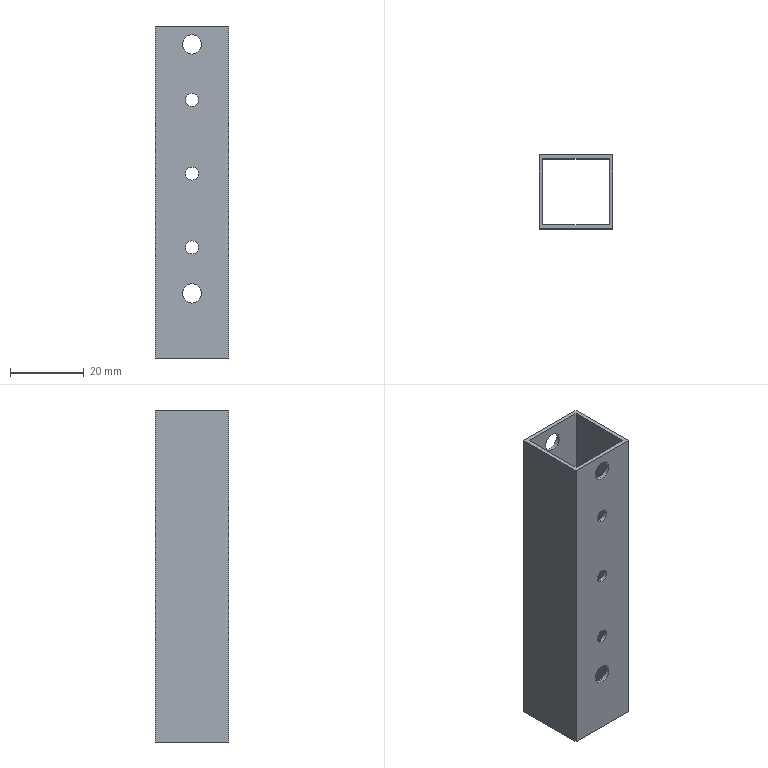Part | SolidWorks | features BaseBody 1 | 1 solid | 30 faces | box 20 x 20 x 90 mm | volume 6697 mm3 | cylinder 20 | plane 10 | commonest cylinder face diameters 3.5 x12 5.2 x8
STEP:
#1=CARTESIAN_POINT('',(0.,9.,68.25));
#2=VERTEX_POINT('',#1);
#3=CARTESIAN_POINT('',(0.,9.,71.75));
#4=VERTEX_POINT('',#3);
#5=CARTESIAN_POINT('',(0.,9.,70.));
#6=DIRECTION('',(0.,1.,0.));
#7=DIRECTION('',(0.,0.,1.));
#8=AXIS2_PLACEMENT_3D('',#5,#6,#7);
#9=CIRCLE('',#8,1.75);
#10=EDGE_CURVE('',#2,#4,#9,.T.);
#11=ORIENTED_EDGE('',*,*,#10,.F.);
#12=CARTESIAN_POINT('',(0.,10.,68.25));
#13=VERTEX_POINT('',#12);
#14=CARTESIAN_POINT('',(0.,-80.,68.25));
#15=DIRECTION('',(0.,1.,0.));
#16=VECTOR('',#15,1000.);
#17=LINE('',#14,#16);
#18=EDGE_CURVE('',#2,#13,#17,.T.);
#19=ORIENTED_EDGE('',*,*,#18,.T.);
#20=CARTESIAN_POINT('',(0.,10.,71.75));
#21=VERTEX_POINT('',#20);
#22=CARTESIAN_POINT('',(0.,10.,70.));
#23=DIRECTION('',(0.,1.,0.));
#24=DIRECTION('',(0.,0.,1.));
#25=AXIS2_PLACEMENT_3D('',#22,#23,#24);
#26=CIRCLE('',#25,1.75);
#27=EDGE_CURVE('',#13,#21,#26,.T.);
#28=ORIENTED_EDGE('',*,*,#27,.T.);
#29=CARTESIAN_POINT('',(0.,-80.,71.75));
#30=DIRECTION('',(0.,1.,0.));
#31=VECTOR('',#30,1000.);
#32=LINE('',#29,#31);
#33=EDGE_CURVE('',#4,#21,#32,.T.);
#34=ORIENTED_EDGE('',*,*,#33,.F.);
#35=EDGE_LOOP('',(#11,#19,#28,#34));
#36=FACE_OUTER_BOUND('',#35,.T.);
#37=CARTESIAN_POINT('',(0.,-80.,70.));
#38=DIRECTION('',(0.,1.,0.));
#39=DIRECTION('',(0.,0.,1.));
#40=AXIS2_PLACEMENT_3D('',#37,#38,#39);
#41=CYLINDRICAL_SURFACE('',#40,1.75);
#42=ADVANCED_FACE('',(#36),#41,.F.);
#43=CARTESIAN_POINT('',(0.,9.,14.9));
#44=VERTEX_POINT('',#43);
#45=CARTESIAN_POINT('',(0.,9.,20.1));
#46=VERTEX_POINT('',#45);
#47=CARTESIAN_POINT('',(0.,9.,17.5));
#48=DIRECTION('',(0.,1.,0.));
#49=DIRECTION('',(0.,0.,1.));
#50=AXIS2_PLACEMENT_3D('',#47,#48,#49);
#51=CIRCLE('',#50,2.6);
#52=EDGE_CURVE('',#44,#46,#51,.T.);
#53=ORIENTED_EDGE('',*,*,#52,.F.);
#54=CARTESIAN_POINT('',(0.,10.,14.9));
#55=VERTEX_POINT('',#54);
#56=CARTESIAN_POINT('',(0.,-80.,14.9));
#57=DIRECTION('',(0.,1.,0.));
#58=VECTOR('',#57,1000.);
#59=LINE('',#56,#58);
#60=EDGE_CURVE('',#44,#55,#59,.T.);
#61=ORIENTED_EDGE('',*,*,#60,.T.);
#62=CARTESIAN_POINT('',(0.,10.,20.1));
#63=VERTEX_POINT('',#62);
#64=CARTESIAN_POINT('',(0.,10.,17.5));
#65=DIRECTION('',(0.,1.,0.));
#66=DIRECTION('',(0.,0.,1.));
#67=AXIS2_PLACEMENT_3D('',#64,#65,#66);
#68=CIRCLE('',#67,2.6);
#69=EDGE_CURVE('',#55,#63,#68,.T.);
#70=ORIENTED_EDGE('',*,*,#69,.T.);
#71=CARTESIAN_POINT('',(0.,-80.,20.1));
#72=DIRECTION('',(0.,1.,0.));
#73=VECTOR('',#72,1000.);
#74=LINE('',#71,#73);
#75=EDGE_CURVE('',#46,#63,#74,.T.);
#76=ORIENTED_EDGE('',*,*,#75,.F.);
#77=EDGE_LOOP('',(#53,#61,#70,#76));
#78=FACE_OUTER_BOUND('',#77,.T.);
#79=CARTESIAN_POINT('',(0.,-80.,17.5));
#80=DIRECTION('',(0.,1.,0.));
#81=DIRECTION('',(0.,0.,1.));
#82=AXIS2_PLACEMENT_3D('',#79,#80,#81);
#83=CYLINDRICAL_SURFACE('',#82,2.6);
#84=ADVANCED_FACE('',(#78),#83,.F.);
#85=CARTESIAN_POINT('',(0.,9.,48.25));
#86=VERTEX_POINT('',#85);
#87=CARTESIAN_POINT('',(0.,9.,51.75));
#88=VERTEX_POINT('',#87);
#89=CARTESIAN_POINT('',(0.,9.,50.));
#90=DIRECTION('',(0.,1.,0.));
#91=DIRECTION('',(0.,0.,1.));
#92=AXIS2_PLACEMENT_3D('',#89,#90,#91);
#93=CIRCLE('',#92,1.75);
#94=EDGE_CURVE('',#86,#88,#93,.T.);
#95=ORIENTED_EDGE('',*,*,#94,.F.);
#96=CARTESIAN_POINT('',(0.,10.,48.25));
#97=VERTEX_POINT('',#96);
#98=CARTESIAN_POINT('',(0.,-80.,48.25));
#99=DIRECTION('',(0.,1.,0.));
#100=VECTOR('',#99,1000.);
#101=LINE('',#98,#100);
#102=EDGE_CURVE('',#86,#97,#101,.T.);
#103=ORIENTED_EDGE('',*,*,#102,.T.);
#104=CARTESIAN_POINT('',(0.,10.,51.75));
#105=VERTEX_POINT('',#104);
#106=CARTESIAN_POINT('',(0.,10.,50.));
#107=DIRECTION('',(0.,1.,0.));
#108=DIRECTION('',(0.,0.,1.));
#109=AXIS2_PLACEMENT_3D('',#106,#107,#108);
#110=CIRCLE('',#109,1.75);
#111=EDGE_CURVE('',#97,#105,#110,.T.);
#112=ORIENTED_EDGE('',*,*,#111,.T.);
#113=CARTESIAN_POINT('',(0.,-80.,51.75));
#114=DIRECTION('',(0.,1.,0.));
#115=VECTOR('',#114,1000.);
#116=LINE('',#113,#115);
#117=EDGE_CURVE('',#88,#105,#116,.T.);
#118=ORIENTED_EDGE('',*,*,#117,.F.);
#119=EDGE_LOOP('',(#95,#103,#112,#118));
#120=FACE_OUTER_BOUND('',#119,.T.);
#121=CARTESIAN_POINT('',(0.,-80.,50.));
#122=DIRECTION('',(0.,1.,0.));
#123=DIRECTION('',(0.,0.,1.));
#124=AXIS2_PLACEMENT_3D('',#121,#122,#123);
#125=CYLINDRICAL_SURFACE('',#124,1.75);
#126=ADVANCED_FACE('',(#120),#125,.F.);
#127=CARTESIAN_POINT('',(0.,9.,28.25));
#128=VERTEX_POINT('',#127);
#129=CARTESIAN_POINT('',(0.,9.,31.75));
#130=VERTEX_POINT('',#129);
#131=CARTESIAN_POINT('',(0.,9.,30.));
#132=DIRECTION('',(0.,1.,0.));
#133=DIRECTION('',(0.,0.,1.));
#134=AXIS2_PLACEMENT_3D('',#131,#132,#133);
#135=CIRCLE('',#134,1.75);
#136=EDGE_CURVE('',#128,#130,#135,.T.);
#137=ORIENTED_EDGE('',*,*,#136,.F.);
#138=CARTESIAN_POINT('',(0.,10.,28.25));
#139=VERTEX_POINT('',#138);
#140=CARTESIAN_POINT('',(0.,-80.,28.25));
#141=DIRECTION('',(0.,1.,0.));
#142=VECTOR('',#141,1000.);
#143=LINE('',#140,#142);
#144=EDGE_CURVE('',#128,#139,#143,.T.);
#145=ORIENTED_EDGE('',*,*,#144,.T.);
#146=CARTESIAN_POINT('',(0.,10.,31.75));
#147=VERTEX_POINT('',#146);
#148=CARTESIAN_POINT('',(0.,10.,30.));
#149=DIRECTION('',(0.,1.,0.));
#150=DIRECTION('',(0.,0.,1.));
#151=AXIS2_PLACEMENT_3D('',#148,#149,#150);
#152=CIRCLE('',#151,1.75);
#153=EDGE_CURVE('',#139,#147,#152,.T.);
#154=ORIENTED_EDGE('',*,*,#153,.T.);
#155=CARTESIAN_POINT('',(0.,-80.,31.75));
#156=DIRECTION('',(0.,1.,0.));
#157=VECTOR('',#156,1000.);
#158=LINE('',#155,#157);
#159=EDGE_CURVE('',#130,#147,#158,.T.);
#160=ORIENTED_EDGE('',*,*,#159,.F.);
#161=EDGE_LOOP('',(#137,#145,#154,#160));
#162=FACE_OUTER_BOUND('',#161,.T.);
#163=CARTESIAN_POINT('',(0.,-80.,30.));
#164=DIRECTION('',(0.,1.,0.));
#165=DIRECTION('',(0.,0.,1.));
#166=AXIS2_PLACEMENT_3D('',#163,#164,#165);
#167=CYLINDRICAL_SURFACE('',#166,1.75);
#168=ADVANCED_FACE('',(#162),#167,.F.);
#169=CARTESIAN_POINT('',(0.,9.,82.4));
#170=VERTEX_POINT('',#169);
#171=CARTESIAN_POINT('',(0.,9.,87.6));
#172=VERTEX_POINT('',#171);
#173=CARTESIAN_POINT('',(0.,9.,85.));
#174=DIRECTION('',(0.,1.,0.));
#175=DIRECTION('',(0.,0.,1.));
#176=AXIS2_PLACEMENT_3D('',#173,#174,#175);
#177=CIRCLE('',#176,2.6);
#178=EDGE_CURVE('',#170,#172,#177,.T.);
#179=ORIENTED_EDGE('',*,*,#178,.F.);
#180=CARTESIAN_POINT('',(0.,10.,82.4));
#181=VERTEX_POINT('',#180);
#182=CARTESIAN_POINT('',(0.,-80.,82.4));
#183=DIRECTION('',(0.,1.,0.));
#184=VECTOR('',#183,1000.);
#185=LINE('',#182,#184);
#186=EDGE_CURVE('',#170,#181,#185,.T.);
#187=ORIENTED_EDGE('',*,*,#186,.T.);
#188=CARTESIAN_POINT('',(0.,10.,87.6));
#189=VERTEX_POINT('',#188);
#190=CARTESIAN_POINT('',(0.,10.,85.));
#191=DIRECTION('',(0.,1.,0.));
#192=DIRECTION('',(0.,0.,1.));
#193=AXIS2_PLACEMENT_3D('',#190,#191,#192);
#194=CIRCLE('',#193,2.6);
#195=EDGE_CURVE('',#181,#189,#194,.T.);
#196=ORIENTED_EDGE('',*,*,#195,.T.);
#197=CARTESIAN_POINT('',(0.,-80.,87.6));
#198=DIRECTION('',(0.,1.,0.));
#199=VECTOR('',#198,1000.);
#200=LINE('',#197,#199);
#201=EDGE_CURVE('',#172,#189,#200,.T.);
#202=ORIENTED_EDGE('',*,*,#201,.F.);
#203=EDGE_LOOP('',(#179,#187,#196,#202));
#204=FACE_OUTER_BOUND('',#203,.T.);
#205=CARTESIAN_POINT('',(0.,-80.,85.));
#206=DIRECTION('',(0.,1.,0.));
#207=DIRECTION('',(0.,0.,1.));
#208=AXIS2_PLACEMENT_3D('',#205,#206,#207);
#209=CYLINDRICAL_SURFACE('',#208,2.6);
#210=ADVANCED_FACE('',(#204),#209,.F.);
#211=CARTESIAN_POINT('',(0.,-10.,71.75));
#212=VERTEX_POINT('',#211);
#213=CARTESIAN_POINT('',(0.,-10.,68.25));
#214=VERTEX_POINT('',#213);
#215=CARTESIAN_POINT('',(0.,-10.,70.));
#216=DIRECTION('',(0.,-1.,0.));
#217=DIRECTION('',(0.,0.,1.));
#218=AXIS2_PLACEMENT_3D('',#215,#216,#217);
#219=CIRCLE('',#218,1.75);
#220=EDGE_CURVE('',#212,#214,#219,.T.);
#221=ORIENTED_EDGE('',*,*,#220,.T.);
#222=CARTESIAN_POINT('',(0.,-9.,68.25));
#223=VERTEX_POINT('',#222);
#224=CARTESIAN_POINT('',(0.,-80.,68.25));
#225=DIRECTION('',(0.,1.,0.));
#226=VECTOR('',#225,1000.);
#227=LINE('',#224,#226);
#228=EDGE_CURVE('',#214,#223,#227,.T.);
#229=ORIENTED_EDGE('',*,*,#228,.T.);
#230=CARTESIAN_POINT('',(0.,-9.,71.75));
#231=VERTEX_POINT('',#230);
#232=CARTESIAN_POINT('',(0.,-9.,70.));
#233=DIRECTION('',(0.,-1.,0.));
#234=DIRECTION('',(0.,0.,1.));
#235=AXIS2_PLACEMENT_3D('',#232,#233,#234);
#236=CIRCLE('',#235,1.75);
#237=EDGE_CURVE('',#231,#223,#236,.T.);
#238=ORIENTED_EDGE('',*,*,#237,.F.);
#239=CARTESIAN_POINT('',(0.,-80.,71.75));
#240=DIRECTION('',(0.,1.,0.));
#241=VECTOR('',#240,1000.);
#242=LINE('',#239,#241);
#243=EDGE_CURVE('',#212,#231,#242,.T.);
#244=ORIENTED_EDGE('',*,*,#243,.F.);
#245=EDGE_LOOP('',(#221,#229,#238,#244));
#246=FACE_OUTER_BOUND('',#245,.T.);
#247=CARTESIAN_POINT('',(0.,-80.,70.));
#248=DIRECTION('',(0.,1.,0.));
#249=DIRECTION('',(0.,0.,1.));
#250=AXIS2_PLACEMENT_3D('',#247,#248,#249);
#251=CYLINDRICAL_SURFACE('',#250,1.75);
#252=ADVANCED_FACE('',(#246),#251,.F.);
#253=CARTESIAN_POINT('',(0.,-10.,20.1));
#254=VERTEX_POINT('',#253);
#255=CARTESIAN_POINT('',(0.,-10.,14.9));
#256=VERTEX_POINT('',#255);
#257=CARTESIAN_POINT('',(0.,-10.,17.5));
#258=DIRECTION('',(0.,-1.,0.));
#259=DIRECTION('',(0.,0.,1.));
#260=AXIS2_PLACEMENT_3D('',#257,#258,#259);
#261=CIRCLE('',#260,2.6);
#262=EDGE_CURVE('',#254,#256,#261,.T.);
#263=ORIENTED_EDGE('',*,*,#262,.T.);
#264=CARTESIAN_POINT('',(0.,-9.,14.9));
#265=VERTEX_POINT('',#264);
#266=CARTESIAN_POINT('',(0.,-80.,14.9));
#267=DIRECTION('',(0.,1.,0.));
#268=VECTOR('',#267,1000.);
#269=LINE('',#266,#268);
#270=EDGE_CURVE('',#256,#265,#269,.T.);
#271=ORIENTED_EDGE('',*,*,#270,.T.);
#272=CARTESIAN_POINT('',(0.,-9.,20.1));
#273=VERTEX_POINT('',#272);
#274=CARTESIAN_POINT('',(0.,-9.,17.5));
#275=DIRECTION('',(0.,-1.,0.));
#276=DIRECTION('',(0.,0.,1.));
#277=AXIS2_PLACEMENT_3D('',#274,#275,#276);
#278=CIRCLE('',#277,2.6);
#279=EDGE_CURVE('',#273,#265,#278,.T.);
#280=ORIENTED_EDGE('',*,*,#279,.F.);
#281=CARTESIAN_POINT('',(0.,-80.,20.1));
#282=DIRECTION('',(0.,1.,0.));
#283=VECTOR('',#282,1000.);
#284=LINE('',#281,#283);
#285=EDGE_CURVE('',#254,#273,#284,.T.);
#286=ORIENTED_EDGE('',*,*,#285,.F.);
#287=EDGE_LOOP('',(#263,#271,#280,#286));
#288=FACE_OUTER_BOUND('',#287,.T.);
#289=CARTESIAN_POINT('',(0.,-80.,17.5));
#290=DIRECTION('',(0.,1.,0.));
#291=DIRECTION('',(0.,0.,1.));
#292=AXIS2_PLACEMENT_3D('',#289,#290,#291);
#293=CYLINDRICAL_SURFACE('',#292,2.6);
#294=ADVANCED_FACE('',(#288),#293,.F.);
#295=CARTESIAN_POINT('',(0.,-10.,51.75));
#296=VERTEX_POINT('',#295);
#297=CARTESIAN_POINT('',(0.,-10.,48.25));
#298=VERTEX_POINT('',#297);
#299=CARTESIAN_POINT('',(0.,-10.,50.));
#300=DIRECTION('',(0.,-1.,0.));
#301=DIRECTION('',(0.,0.,1.));
#302=AXIS2_PLACEMENT_3D('',#299,#300,#301);
#303=CIRCLE('',#302,1.75);
#304=EDGE_CURVE('',#296,#298,#303,.T.);
#305=ORIENTED_EDGE('',*,*,#304,.T.);
#306=CARTESIAN_POINT('',(0.,-9.,48.25));
#307=VERTEX_POINT('',#306);
#308=CARTESIAN_POINT('',(0.,-80.,48.25));
#309=DIRECTION('',(0.,1.,0.));
#310=VECTOR('',#309,1000.);
#311=LINE('',#308,#310);
#312=EDGE_CURVE('',#298,#307,#311,.T.);
#313=ORIENTED_EDGE('',*,*,#312,.T.);
#314=CARTESIAN_POINT('',(0.,-9.,51.75));
#315=VERTEX_POINT('',#314);
#316=CARTESIAN_POINT('',(0.,-9.,50.));
#317=DIRECTION('',(0.,-1.,0.));
#318=DIRECTION('',(0.,0.,1.));
#319=AXIS2_PLACEMENT_3D('',#316,#317,#318);
#320=CIRCLE('',#319,1.75);
#321=EDGE_CURVE('',#315,#307,#320,.T.);
#322=ORIENTED_EDGE('',*,*,#321,.F.);
#323=CARTESIAN_POINT('',(0.,-80.,51.75));
#324=DIRECTION('',(0.,1.,0.));
#325=VECTOR('',#324,1000.);
#326=LINE('',#323,#325);
#327=EDGE_CURVE('',#296,#315,#326,.T.);
#328=ORIENTED_EDGE('',*,*,#327,.F.);
#329=EDGE_LOOP('',(#305,#313,#322,#328));
#330=FACE_OUTER_BOUND('',#329,.T.);
#331=CARTESIAN_POINT('',(0.,-80.,50.));
#332=DIRECTION('',(0.,1.,0.));
#333=DIRECTION('',(0.,0.,1.));
#334=AXIS2_PLACEMENT_3D('',#331,#332,#333);
#335=CYLINDRICAL_SURFACE('',#334,1.75);
#336=ADVANCED_FACE('',(#330),#335,.F.);
#337=CARTESIAN_POINT('',(0.,-10.,31.75));
#338=VERTEX_POINT('',#337);
#339=CARTESIAN_POINT('',(0.,-10.,28.25));
#340=VERTEX_POINT('',#339);
#341=CARTESIAN_POINT('',(0.,-10.,30.));
#342=DIRECTION('',(0.,-1.,0.));
#343=DIRECTION('',(0.,0.,1.));
#344=AXIS2_PLACEMENT_3D('',#341,#342,#343);
#345=CIRCLE('',#344,1.75);
#346=EDGE_CURVE('',#338,#340,#345,.T.);
#347=ORIENTED_EDGE('',*,*,#346,.T.);
#348=CARTESIAN_POINT('',(0.,-9.,28.25));
#349=VERTEX_POINT('',#348);
#350=CARTESIAN_POINT('',(0.,-80.,28.25));
#351=DIRECTION('',(0.,1.,0.));
#352=VECTOR('',#351,1000.);
#353=LINE('',#350,#352);
#354=EDGE_CURVE('',#340,#349,#353,.T.);
#355=ORIENTED_EDGE('',*,*,#354,.T.);
#356=CARTESIAN_POINT('',(0.,-9.,31.75));
#357=VERTEX_POINT('',#356);
#358=CARTESIAN_POINT('',(0.,-9.,30.));
#359=DIRECTION('',(0.,-1.,0.));
#360=DIRECTION('',(0.,0.,1.));
#361=AXIS2_PLACEMENT_3D('',#358,#359,#360);
#362=CIRCLE('',#361,1.75);
#363=EDGE_CURVE('',#357,#349,#362,.T.);
#364=ORIENTED_EDGE('',*,*,#363,.F.);
#365=CARTESIAN_POINT('',(0.,-80.,31.75));
#366=DIRECTION('',(0.,1.,0.));
#367=VECTOR('',#366,1000.);
#368=LINE('',#365,#367);
#369=EDGE_CURVE('',#338,#357,#368,.T.);
#370=ORIENTED_EDGE('',*,*,#369,.F.);
#371=EDGE_LOOP('',(#347,#355,#364,#370));
#372=FACE_OUTER_BOUND('',#371,.T.);
#373=CARTESIAN_POINT('',(0.,-80.,30.));
#374=DIRECTION('',(0.,1.,0.));
#375=DIRECTION('',(0.,0.,1.));
#376=AXIS2_PLACEMENT_3D('',#373,#374,#375);
#377=CYLINDRICAL_SURFACE('',#376,1.75);
#378=ADVANCED_FACE('',(#372),#377,.F.);
#379=CARTESIAN_POINT('',(0.,-10.,87.6));
#380=VERTEX_POINT('',#379);
#381=CARTESIAN_POINT('',(0.,-10.,82.4));
#382=VERTEX_POINT('',#381);
#383=CARTESIAN_POINT('',(0.,-10.,85.));
#384=DIRECTION('',(0.,-1.,0.));
#385=DIRECTION('',(0.,0.,1.));
#386=AXIS2_PLACEMENT_3D('',#383,#384,#385);
#387=CIRCLE('',#386,2.6);
#388=EDGE_CURVE('',#380,#382,#387,.T.);
#389=ORIENTED_EDGE('',*,*,#388,.T.);
#390=CARTESIAN_POINT('',(0.,-9.,82.4));
#391=VERTEX_POINT('',#390);
#392=CARTESIAN_POINT('',(0.,-80.,82.4));
#393=DIRECTION('',(0.,1.,0.));
#394=VECTOR('',#393,1000.);
#395=LINE('',#392,#394);
#396=EDGE_CURVE('',#382,#391,#395,.T.);
#397=ORIENTED_EDGE('',*,*,#396,.T.);
#398=CARTESIAN_POINT('',(0.,-9.,87.6));
#399=VERTEX_POINT('',#398);
#400=CARTESIAN_POINT('',(0.,-9.,85.));
#401=DIRECTION('',(0.,-1.,0.));
#402=DIRECTION('',(0.,0.,1.));
#403=AXIS2_PLACEMENT_3D('',#400,#401,#402);
#404=CIRCLE('',#403,2.6);
#405=EDGE_CURVE('',#399,#391,#404,.T.);
#406=ORIENTED_EDGE('',*,*,#405,.F.);
#407=CARTESIAN_POINT('',(0.,-80.,87.6));
#408=DIRECTION('',(0.,1.,0.));
#409=VECTOR('',#408,1000.);
#410=LINE('',#407,#409);
#411=EDGE_CURVE('',#380,#399,#410,.T.);
#412=ORIENTED_EDGE('',*,*,#411,.F.);
#413=EDGE_LOOP('',(#389,#397,#406,#412));
#414=FACE_OUTER_BOUND('',#413,.T.);
#415=CARTESIAN_POINT('',(0.,-80.,85.));
#416=DIRECTION('',(0.,1.,0.));
#417=DIRECTION('',(0.,0.,1.));
#418=AXIS2_PLACEMENT_3D('',#415,#416,#417);
#419=CYLINDRICAL_SURFACE('',#418,2.6);
#420=ADVANCED_FACE('',(#414),#419,.F.);
#421=CARTESIAN_POINT('',(10.,10.,90.));
#422=VERTEX_POINT('',#421);
#423=CARTESIAN_POINT('',(10.,10.,0.));
#424=VERTEX_POINT('',#423);
#425=CARTESIAN_POINT('',(10.,10.,90.));
#426=DIRECTION('',(0.,0.,-1.));
#427=VECTOR('',#426,1000.);
#428=LINE('',#425,#427);
#429=EDGE_CURVE('',#422,#424,#428,.T.);
#430=ORIENTED_EDGE('',*,*,#429,.F.);
#431=CARTESIAN_POINT('',(10.,-10.,90.));
#432=VERTEX_POINT('',#431);
#433=CARTESIAN_POINT('',(10.,10.,90.));
#434=DIRECTION('',(0.,1.,0.));
#435=VECTOR('',#434,1000.);
#436=LINE('',#433,#435);
#437=EDGE_CURVE('',#432,#422,#436,.T.);
#438=ORIENTED_EDGE('',*,*,#437,.F.);
#439=CARTESIAN_POINT('',(10.,-10.,0.));
#440=VERTEX_POINT('',#439);
#441=CARTESIAN_POINT('',(10.,-10.,90.));
#442=DIRECTION('',(0.,0.,1.));
#443=VECTOR('',#442,1000.);
#444=LINE('',#441,#443);
#445=EDGE_CURVE('',#440,#432,#444,.T.);
#446=ORIENTED_EDGE('',*,*,#445,.F.);
#447=CARTESIAN_POINT('',(10.,10.,0.));
#448=DIRECTION('',(0.,-1.,0.));
#449=VECTOR('',#448,1000.);
#450=LINE('',#447,#449);
#451=EDGE_CURVE('',#424,#440,#450,.T.);
#452=ORIENTED_EDGE('',*,*,#451,.F.);
#453=EDGE_LOOP('',(#430,#438,#446,#452));
#454=FACE_OUTER_BOUND('',#453,.T.);
#455=CARTESIAN_POINT('',(10.,10.,90.));
#456=DIRECTION('',(-1.,0.,0.));
#457=DIRECTION('',(0.,-1.,0.));
#458=AXIS2_PLACEMENT_3D('',#455,#456,#457);
#459=PLANE('',#458);
#460=ADVANCED_FACE('',(#454),#459,.F.);
#461=CARTESIAN_POINT('',(-9.,9.,0.));
#462=VERTEX_POINT('',#461);
#463=CARTESIAN_POINT('',(9.,9.,0.));
#464=VERTEX_POINT('',#463);
#465=CARTESIAN_POINT('',(0.,9.,0.));
#466=DIRECTION('',(1.,0.,0.));
#467=VECTOR('',#466,1000.);
#468=LINE('',#465,#467);
#469=EDGE_CURVE('',#462,#464,#468,.T.);
#470=ORIENTED_EDGE('',*,*,#469,.F.);
#471=CARTESIAN_POINT('',(-9.,-9.,0.));
#472=VERTEX_POINT('',#471);
#473=CARTESIAN_POINT('',(-9.,0.,0.));
#474=DIRECTION('',(0.,1.,0.));
#475=VECTOR('',#474,1000.);
#476=LINE('',#473,#475);
#477=EDGE_CURVE('',#472,#462,#476,.T.);
#478=ORIENTED_EDGE('',*,*,#477,.F.);
#479=CARTESIAN_POINT('',(9.,-9.,0.));
#480=VERTEX_POINT('',#479);
#481=CARTESIAN_POINT('',(0.,-9.,0.));
#482=DIRECTION('',(-1.,0.,0.));
#483=VECTOR('',#482,1000.);
#484=LINE('',#481,#483);
#485=EDGE_CURVE('',#480,#472,#484,.T.);
#486=ORIENTED_EDGE('',*,*,#485,.F.);
#487=CARTESIAN_POINT('',(9.,0.,0.));
#488=DIRECTION('',(0.,-1.,0.));
#489=VECTOR('',#488,1000.);
#490=LINE('',#487,#489);
#491=EDGE_CURVE('',#464,#480,#490,.T.);
#492=ORIENTED_EDGE('',*,*,#491,.F.);
#493=EDGE_LOOP('',(#470,#478,#486,#492));
#494=FACE_BOUND('',#493,.T.);
#495=CARTESIAN_POINT('',(-10.,-10.,0.));
#496=VERTEX_POINT('',#495);
#497=CARTESIAN_POINT('',(0.,-10.,0.));
#498=DIRECTION('',(1.,0.,0.));
#499=VECTOR('',#498,1000.);
#500=LINE('',#497,#499);
#501=EDGE_CURVE('',#496,#440,#500,.T.);
#502=ORIENTED_EDGE('',*,*,#501,.F.);
#503=CARTESIAN_POINT('',(-10.,10.,0.));
#504=VERTEX_POINT('',#503);
#505=CARTESIAN_POINT('',(-10.,0.,0.));
#506=DIRECTION('',(0.,-1.,0.));
#507=VECTOR('',#506,1000.);
#508=LINE('',#505,#507);
#509=EDGE_CURVE('',#504,#496,#508,.T.);
#510=ORIENTED_EDGE('',*,*,#509,.F.);
#511=CARTESIAN_POINT('',(0.,10.,0.));
#512=DIRECTION('',(-1.,0.,0.));
#513=VECTOR('',#512,1000.);
#514=LINE('',#511,#513);
#515=EDGE_CURVE('',#424,#504,#514,.T.);
#516=ORIENTED_EDGE('',*,*,#515,.F.);
#517=ORIENTED_EDGE('',*,*,#451,.T.);
#518=EDGE_LOOP('',(#502,#510,#516,#517));
#519=FACE_OUTER_BOUND('',#518,.T.);
#520=CARTESIAN_POINT('',(0.,0.,0.));
#521=DIRECTION('',(0.,0.,1.));
#522=DIRECTION('',(1.,0.,0.));
#523=AXIS2_PLACEMENT_3D('',#520,#521,#522);
#524=PLANE('',#523);
#525=ADVANCED_FACE('',(#494,#519),#524,.F.);
#526=CARTESIAN_POINT('',(-10.,10.,90.));
#527=VERTEX_POINT('',#526);
#528=CARTESIAN_POINT('',(-10.,10.,90.));
#529=DIRECTION('',(0.,0.,-1.));
#530=VECTOR('',#529,1000.);
#531=LINE('',#528,#530);
#532=EDGE_CURVE('',#527,#504,#531,.T.);
#533=ORIENTED_EDGE('',*,*,#532,.F.);
#534=CARTESIAN_POINT('',(-10.,10.,90.));
#535=DIRECTION('',(-1.,0.,0.));
#536=VECTOR('',#535,1000.);
#537=LINE('',#534,#536);
#538=EDGE_CURVE('',#422,#527,#537,.T.);
#539=ORIENTED_EDGE('',*,*,#538,.F.);
#540=ORIENTED_EDGE('',*,*,#429,.T.);
#541=ORIENTED_EDGE('',*,*,#515,.T.);
#542=EDGE_LOOP('',(#533,#539,#540,#541));
#543=FACE_OUTER_BOUND('',#542,.T.);
#544=CARTESIAN_POINT('',(0.,10.,70.));
#545=DIRECTION('',(0.,1.,0.));
#546=DIRECTION('',(0.,0.,1.));
#547=AXIS2_PLACEMENT_3D('',#544,#545,#546);
#548=CIRCLE('',#547,1.75);
#549=EDGE_CURVE('',#21,#13,#548,.T.);
#550=ORIENTED_EDGE('',*,*,#549,.F.);
#551=ORIENTED_EDGE('',*,*,#27,.F.);
#552=EDGE_LOOP('',(#550,#551));
#553=FACE_BOUND('',#552,.T.);
#554=CARTESIAN_POINT('',(0.,10.,17.5));
#555=DIRECTION('',(0.,1.,0.));
#556=DIRECTION('',(0.,0.,1.));
#557=AXIS2_PLACEMENT_3D('',#554,#555,#556);
#558=CIRCLE('',#557,2.6);
#559=EDGE_CURVE('',#63,#55,#558,.T.);
#560=ORIENTED_EDGE('',*,*,#559,.F.);
#561=ORIENTED_EDGE('',*,*,#69,.F.);
#562=EDGE_LOOP('',(#560,#561));
#563=FACE_BOUND('',#562,.T.);
#564=CARTESIAN_POINT('',(0.,10.,50.));
#565=DIRECTION('',(0.,1.,0.));
#566=DIRECTION('',(0.,0.,1.));
#567=AXIS2_PLACEMENT_3D('',#564,#565,#566);
#568=CIRCLE('',#567,1.75);
#569=EDGE_CURVE('',#105,#97,#568,.T.);
#570=ORIENTED_EDGE('',*,*,#569,.F.);
#571=ORIENTED_EDGE('',*,*,#111,.F.);
#572=EDGE_LOOP('',(#570,#571));
#573=FACE_BOUND('',#572,.T.);
#574=CARTESIAN_POINT('',(0.,10.,30.));
#575=DIRECTION('',(0.,1.,0.));
#576=DIRECTION('',(0.,0.,1.));
#577=AXIS2_PLACEMENT_3D('',#574,#575,#576);
#578=CIRCLE('',#577,1.75);
#579=EDGE_CURVE('',#147,#139,#578,.T.);
#580=ORIENTED_EDGE('',*,*,#579,.F.);
#581=ORIENTED_EDGE('',*,*,#153,.F.);
#582=EDGE_LOOP('',(#580,#581));
#583=FACE_BOUND('',#582,.T.);
#584=CARTESIAN_POINT('',(0.,10.,85.));
#585=DIRECTION('',(0.,1.,0.));
#586=DIRECTION('',(0.,0.,1.));
#587=AXIS2_PLACEMENT_3D('',#584,#585,#586);
#588=CIRCLE('',#587,2.6);
#589=EDGE_CURVE('',#189,#181,#588,.T.);
#590=ORIENTED_EDGE('',*,*,#589,.F.);
#591=ORIENTED_EDGE('',*,*,#195,.F.);
#592=EDGE_LOOP('',(#590,#591));
#593=FACE_BOUND('',#592,.T.);
#594=CARTESIAN_POINT('',(-10.,10.,90.));
#595=DIRECTION('',(0.,-1.,0.));
#596=DIRECTION('',(0.,0.,-1.));
#597=AXIS2_PLACEMENT_3D('',#594,#595,#596);
#598=PLANE('',#597);
#599=ADVANCED_FACE('',(#543,#553,#563,#573,#583,#593),#598,.F.);
#600=CARTESIAN_POINT('',(9.,-9.,90.));
#601=VERTEX_POINT('',#600);
#602=CARTESIAN_POINT('',(-9.,-9.,90.));
#603=VERTEX_POINT('',#602);
#604=CARTESIAN_POINT('',(0.,-9.,90.));
#605=DIRECTION('',(-1.,0.,0.));
#606=VECTOR('',#605,1000.);
#607=LINE('',#604,#606);
#608=EDGE_CURVE('',#601,#603,#607,.T.);
#609=ORIENTED_EDGE('',*,*,#608,.T.);
#610=CARTESIAN_POINT('',(-9.,9.,90.));
#611=VERTEX_POINT('',#610);
#612=CARTESIAN_POINT('',(-9.,0.,90.));
#613=DIRECTION('',(0.,1.,0.));
#614=VECTOR('',#613,1000.);
#615=LINE('',#612,#614);
#616=EDGE_CURVE('',#603,#611,#615,.T.);
#617=ORIENTED_EDGE('',*,*,#616,.T.);
#618=CARTESIAN_POINT('',(9.,9.,90.));
#619=VERTEX_POINT('',#618);
#620=CARTESIAN_POINT('',(0.,9.,90.));
#621=DIRECTION('',(1.,0.,0.));
#622=VECTOR('',#621,1000.);
#623=LINE('',#620,#622);
#624=EDGE_CURVE('',#611,#619,#623,.T.);
#625=ORIENTED_EDGE('',*,*,#624,.T.);
#626=CARTESIAN_POINT('',(9.,0.,90.));
#627=DIRECTION('',(0.,-1.,0.));
#628=VECTOR('',#627,1000.);
#629=LINE('',#626,#628);
#630=EDGE_CURVE('',#619,#601,#629,.T.);
#631=ORIENTED_EDGE('',*,*,#630,.T.);
#632=EDGE_LOOP('',(#609,#617,#625,#631));
#633=FACE_BOUND('',#632,.T.);
#634=CARTESIAN_POINT('',(-10.,-10.,90.));
#635=VERTEX_POINT('',#634);
#636=CARTESIAN_POINT('',(-10.,0.,90.));
#637=DIRECTION('',(0.,-1.,0.));
#638=VECTOR('',#637,1000.);
#639=LINE('',#636,#638);
#640=EDGE_CURVE('',#527,#635,#639,.T.);
#641=ORIENTED_EDGE('',*,*,#640,.T.);
#642=CARTESIAN_POINT('',(0.,-10.,90.));
#643=DIRECTION('',(1.,0.,0.));
#644=VECTOR('',#643,1000.);
#645=LINE('',#642,#644);
#646=EDGE_CURVE('',#635,#432,#645,.T.);
#647=ORIENTED_EDGE('',*,*,#646,.T.);
#648=ORIENTED_EDGE('',*,*,#437,.T.);
#649=ORIENTED_EDGE('',*,*,#538,.T.);
#650=EDGE_LOOP('',(#641,#647,#648,#649));
#651=FACE_OUTER_BOUND('',#650,.T.);
#652=CARTESIAN_POINT('',(0.,0.,90.));
#653=DIRECTION('',(0.,0.,1.));
#654=DIRECTION('',(1.,0.,0.));
#655=AXIS2_PLACEMENT_3D('',#652,#653,#654);
#656=PLANE('',#655);
#657=ADVANCED_FACE('',(#633,#651),#656,.T.);
#658=ORIENTED_EDGE('',*,*,#445,.T.);
#659=ORIENTED_EDGE('',*,*,#646,.F.);
#660=CARTESIAN_POINT('',(-10.,-10.,90.));
#661=DIRECTION('',(0.,0.,1.));
#662=VECTOR('',#661,1000.);
#663=LINE('',#660,#662);
#664=EDGE_CURVE('',#496,#635,#663,.T.);
#665=ORIENTED_EDGE('',*,*,#664,.F.);
#666=ORIENTED_EDGE('',*,*,#501,.T.);
#667=EDGE_LOOP('',(#658,#659,#665,#666));
#668=FACE_OUTER_BOUND('',#667,.T.);
#669=ORIENTED_EDGE('',*,*,#220,.F.);
#670=CARTESIAN_POINT('',(0.,-10.,70.));
#671=DIRECTION('',(0.,-1.,0.));
#672=DIRECTION('',(0.,0.,1.));
#673=AXIS2_PLACEMENT_3D('',#670,#671,#672);
#674=CIRCLE('',#673,1.75);
#675=EDGE_CURVE('',#214,#212,#674,.T.);
#676=ORIENTED_EDGE('',*,*,#675,.F.);
#677=EDGE_LOOP('',(#669,#676));
#678=FACE_BOUND('',#677,.T.);
#679=ORIENTED_EDGE('',*,*,#262,.F.);
#680=CARTESIAN_POINT('',(0.,-10.,17.5));
#681=DIRECTION('',(0.,-1.,0.));
#682=DIRECTION('',(0.,0.,1.));
#683=AXIS2_PLACEMENT_3D('',#680,#681,#682);
#684=CIRCLE('',#683,2.6);
#685=EDGE_CURVE('',#256,#254,#684,.T.);
#686=ORIENTED_EDGE('',*,*,#685,.F.);
#687=EDGE_LOOP('',(#679,#686));
#688=FACE_BOUND('',#687,.T.);
#689=ORIENTED_EDGE('',*,*,#304,.F.);
#690=CARTESIAN_POINT('',(0.,-10.,50.));
#691=DIRECTION('',(0.,-1.,0.));
#692=DIRECTION('',(0.,0.,1.));
#693=AXIS2_PLACEMENT_3D('',#690,#691,#692);
#694=CIRCLE('',#693,1.75);
#695=EDGE_CURVE('',#298,#296,#694,.T.);
#696=ORIENTED_EDGE('',*,*,#695,.F.);
#697=EDGE_LOOP('',(#689,#696));
#698=FACE_BOUND('',#697,.T.);
#699=ORIENTED_EDGE('',*,*,#346,.F.);
#700=CARTESIAN_POINT('',(0.,-10.,30.));
#701=DIRECTION('',(0.,-1.,0.));
#702=DIRECTION('',(0.,0.,1.));
#703=AXIS2_PLACEMENT_3D('',#700,#701,#702);
#704=CIRCLE('',#703,1.75);
#705=EDGE_CURVE('',#340,#338,#704,.T.);
#706=ORIENTED_EDGE('',*,*,#705,.F.);
#707=EDGE_LOOP('',(#699,#706));
#708=FACE_BOUND('',#707,.T.);
#709=ORIENTED_EDGE('',*,*,#388,.F.);
#710=CARTESIAN_POINT('',(0.,-10.,85.));
#711=DIRECTION('',(0.,-1.,0.));
#712=DIRECTION('',(0.,0.,1.));
#713=AXIS2_PLACEMENT_3D('',#710,#711,#712);
#714=CIRCLE('',#713,2.6);
#715=EDGE_CURVE('',#382,#380,#714,.T.);
#716=ORIENTED_EDGE('',*,*,#715,.F.);
#717=EDGE_LOOP('',(#709,#716));
#718=FACE_BOUND('',#717,.T.);
#719=CARTESIAN_POINT('',(-10.,-10.,90.));
#720=DIRECTION('',(0.,1.,0.));
#721=DIRECTION('',(0.,0.,1.));
#722=AXIS2_PLACEMENT_3D('',#719,#720,#721);
#723=PLANE('',#722);
#724=ADVANCED_FACE('',(#668,#678,#688,#698,#708,#718),#723,.F.);
#725=ORIENTED_EDGE('',*,*,#630,.F.);
#726=CARTESIAN_POINT('',(9.,9.,90.));
#727=DIRECTION('',(0.,0.,-1.));
#728=VECTOR('',#727,1000.);
#729=LINE('',#726,#728);
#730=EDGE_CURVE('',#619,#464,#729,.T.);
#731=ORIENTED_EDGE('',*,*,#730,.T.);
#732=ORIENTED_EDGE('',*,*,#491,.T.);
#733=CARTESIAN_POINT('',(9.,-9.,90.));
#734=DIRECTION('',(0.,0.,1.));
#735=VECTOR('',#734,1000.);
#736=LINE('',#733,#735);
#737=EDGE_CURVE('',#480,#601,#736,.T.);
#738=ORIENTED_EDGE('',*,*,#737,.T.);
#739=EDGE_LOOP('',(#725,#731,#732,#738));
#740=FACE_OUTER_BOUND('',#739,.T.);
#741=CARTESIAN_POINT('',(9.,9.,90.));
#742=DIRECTION('',(-1.,0.,0.));
#743=DIRECTION('',(0.,0.,1.));
#744=AXIS2_PLACEMENT_3D('',#741,#742,#743);
#745=PLANE('',#744);
#746=ADVANCED_FACE('',(#740),#745,.T.);
#747=ORIENTED_EDGE('',*,*,#624,.F.);
#748=CARTESIAN_POINT('',(-9.,9.,90.));
#749=DIRECTION('',(0.,0.,-1.));
#750=VECTOR('',#749,1000.);
#751=LINE('',#748,#750);
#752=EDGE_CURVE('',#611,#462,#751,.T.);
#753=ORIENTED_EDGE('',*,*,#752,.T.);
#754=ORIENTED_EDGE('',*,*,#469,.T.);
#755=ORIENTED_EDGE('',*,*,#730,.F.);
#756=EDGE_LOOP('',(#747,#753,#754,#755));
#757=FACE_OUTER_BOUND('',#756,.T.);
#758=CARTESIAN_POINT('',(0.,9.,70.));
#759=DIRECTION('',(0.,1.,0.));
#760=DIRECTION('',(0.,0.,1.));
#761=AXIS2_PLACEMENT_3D('',#758,#759,#760);
#762=CIRCLE('',#761,1.75);
#763=EDGE_CURVE('',#4,#2,#762,.T.);
#764=ORIENTED_EDGE('',*,*,#763,.T.);
#765=ORIENTED_EDGE('',*,*,#10,.T.);
#766=EDGE_LOOP('',(#764,#765));
#767=FACE_BOUND('',#766,.T.);
#768=CARTESIAN_POINT('',(0.,9.,17.5));
#769=DIRECTION('',(0.,1.,0.));
#770=DIRECTION('',(0.,0.,1.));
#771=AXIS2_PLACEMENT_3D('',#768,#769,#770);
#772=CIRCLE('',#771,2.6);
#773=EDGE_CURVE('',#46,#44,#772,.T.);
#774=ORIENTED_EDGE('',*,*,#773,.T.);
#775=ORIENTED_EDGE('',*,*,#52,.T.);
#776=EDGE_LOOP('',(#774,#775));
#777=FACE_BOUND('',#776,.T.);
#778=CARTESIAN_POINT('',(0.,9.,50.));
#779=DIRECTION('',(0.,1.,0.));
#780=DIRECTION('',(0.,0.,1.));
#781=AXIS2_PLACEMENT_3D('',#778,#779,#780);
#782=CIRCLE('',#781,1.75);
#783=EDGE_CURVE('',#88,#86,#782,.T.);
#784=ORIENTED_EDGE('',*,*,#783,.T.);
#785=ORIENTED_EDGE('',*,*,#94,.T.);
#786=EDGE_LOOP('',(#784,#785));
#787=FACE_BOUND('',#786,.T.);
#788=CARTESIAN_POINT('',(0.,9.,30.));
#789=DIRECTION('',(0.,1.,0.));
#790=DIRECTION('',(0.,0.,1.));
#791=AXIS2_PLACEMENT_3D('',#788,#789,#790);
#792=CIRCLE('',#791,1.75);
#793=EDGE_CURVE('',#130,#128,#792,.T.);
#794=ORIENTED_EDGE('',*,*,#793,.T.);
#795=ORIENTED_EDGE('',*,*,#136,.T.);
#796=EDGE_LOOP('',(#794,#795));
#797=FACE_BOUND('',#796,.T.);
#798=CARTESIAN_POINT('',(0.,9.,85.));
#799=DIRECTION('',(0.,1.,0.));
#800=DIRECTION('',(0.,0.,1.));
#801=AXIS2_PLACEMENT_3D('',#798,#799,#800);
#802=CIRCLE('',#801,2.6);
#803=EDGE_CURVE('',#172,#170,#802,.T.);
#804=ORIENTED_EDGE('',*,*,#803,.T.);
#805=ORIENTED_EDGE('',*,*,#178,.T.);
#806=EDGE_LOOP('',(#804,#805));
#807=FACE_BOUND('',#806,.T.);
#808=CARTESIAN_POINT('',(-9.,9.,90.));
#809=DIRECTION('',(0.,-1.,0.));
#810=DIRECTION('',(0.,0.,-1.));
#811=AXIS2_PLACEMENT_3D('',#808,#809,#810);
#812=PLANE('',#811);
#813=ADVANCED_FACE('',(#757,#767,#777,#787,#797,#807),#812,.T.);
#814=ORIENTED_EDGE('',*,*,#616,.F.);
#815=CARTESIAN_POINT('',(-9.,-9.,90.));
#816=DIRECTION('',(0.,0.,-1.));
#817=VECTOR('',#816,1000.);
#818=LINE('',#815,#817);
#819=EDGE_CURVE('',#603,#472,#818,.T.);
#820=ORIENTED_EDGE('',*,*,#819,.T.);
#821=ORIENTED_EDGE('',*,*,#477,.T.);
#822=ORIENTED_EDGE('',*,*,#752,.F.);
#823=EDGE_LOOP('',(#814,#820,#821,#822));
#824=FACE_OUTER_BOUND('',#823,.T.);
#825=CARTESIAN_POINT('',(-9.,9.,90.));
#826=DIRECTION('',(1.,0.,0.));
#827=DIRECTION('',(0.,0.,-1.));
#828=AXIS2_PLACEMENT_3D('',#825,#826,#827);
#829=PLANE('',#828);
#830=ADVANCED_FACE('',(#824),#829,.T.);
#831=ORIENTED_EDGE('',*,*,#608,.F.);
#832=ORIENTED_EDGE('',*,*,#737,.F.);
#833=ORIENTED_EDGE('',*,*,#485,.T.);
#834=ORIENTED_EDGE('',*,*,#819,.F.);
#835=EDGE_LOOP('',(#831,#832,#833,#834));
#836=FACE_OUTER_BOUND('',#835,.T.);
#837=ORIENTED_EDGE('',*,*,#237,.T.);
#838=CARTESIAN_POINT('',(0.,-9.,70.));
#839=DIRECTION('',(0.,-1.,0.));
#840=DIRECTION('',(0.,0.,1.));
#841=AXIS2_PLACEMENT_3D('',#838,#839,#840);
#842=CIRCLE('',#841,1.75);
#843=EDGE_CURVE('',#223,#231,#842,.T.);
#844=ORIENTED_EDGE('',*,*,#843,.T.);
#845=EDGE_LOOP('',(#837,#844));
#846=FACE_BOUND('',#845,.T.);
#847=ORIENTED_EDGE('',*,*,#279,.T.);
#848=CARTESIAN_POINT('',(0.,-9.,17.5));
#849=DIRECTION('',(0.,-1.,0.));
#850=DIRECTION('',(0.,0.,1.));
#851=AXIS2_PLACEMENT_3D('',#848,#849,#850);
#852=CIRCLE('',#851,2.6);
#853=EDGE_CURVE('',#265,#273,#852,.T.);
#854=ORIENTED_EDGE('',*,*,#853,.T.);
#855=EDGE_LOOP('',(#847,#854));
#856=FACE_BOUND('',#855,.T.);
#857=ORIENTED_EDGE('',*,*,#321,.T.);
#858=CARTESIAN_POINT('',(0.,-9.,50.));
#859=DIRECTION('',(0.,-1.,0.));
#860=DIRECTION('',(0.,0.,1.));
#861=AXIS2_PLACEMENT_3D('',#858,#859,#860);
#862=CIRCLE('',#861,1.75);
#863=EDGE_CURVE('',#307,#315,#862,.T.);
#864=ORIENTED_EDGE('',*,*,#863,.T.);
#865=EDGE_LOOP('',(#857,#864));
#866=FACE_BOUND('',#865,.T.);
#867=ORIENTED_EDGE('',*,*,#363,.T.);
#868=CARTESIAN_POINT('',(0.,-9.,30.));
#869=DIRECTION('',(0.,-1.,0.));
#870=DIRECTION('',(0.,0.,1.));
#871=AXIS2_PLACEMENT_3D('',#868,#869,#870);
#872=CIRCLE('',#871,1.75);
#873=EDGE_CURVE('',#349,#357,#872,.T.);
#874=ORIENTED_EDGE('',*,*,#873,.T.);
#875=EDGE_LOOP('',(#867,#874));
#876=FACE_BOUND('',#875,.T.);
#877=ORIENTED_EDGE('',*,*,#405,.T.);
#878=CARTESIAN_POINT('',(0.,-9.,85.));
#879=DIRECTION('',(0.,-1.,0.));
#880=DIRECTION('',(0.,0.,1.));
#881=AXIS2_PLACEMENT_3D('',#878,#879,#880);
#882=CIRCLE('',#881,2.6);
#883=EDGE_CURVE('',#391,#399,#882,.T.);
#884=ORIENTED_EDGE('',*,*,#883,.T.);
#885=EDGE_LOOP('',(#877,#884));
#886=FACE_BOUND('',#885,.T.);
#887=CARTESIAN_POINT('',(-9.,-9.,90.));
#888=DIRECTION('',(0.,1.,0.));
#889=DIRECTION('',(0.,0.,1.));
#890=AXIS2_PLACEMENT_3D('',#887,#888,#889);
#891=PLANE('',#890);
#892=ADVANCED_FACE('',(#836,#846,#856,#866,#876,#886),#891,.T.);
#893=ORIENTED_EDGE('',*,*,#664,.T.);
#894=ORIENTED_EDGE('',*,*,#640,.F.);
#895=ORIENTED_EDGE('',*,*,#532,.T.);
#896=ORIENTED_EDGE('',*,*,#509,.T.);
#897=EDGE_LOOP('',(#893,#894,#895,#896));
#898=FACE_OUTER_BOUND('',#897,.T.);
#899=CARTESIAN_POINT('',(-10.,10.,90.));
#900=DIRECTION('',(1.,0.,0.));
#901=DIRECTION('',(0.,1.,0.));
#902=AXIS2_PLACEMENT_3D('',#899,#900,#901);
#903=PLANE('',#902);
#904=ADVANCED_FACE('',(#898),#903,.F.);
#905=ORIENTED_EDGE('',*,*,#18,.F.);
#906=ORIENTED_EDGE('',*,*,#763,.F.);
#907=ORIENTED_EDGE('',*,*,#33,.T.);
#908=ORIENTED_EDGE('',*,*,#549,.T.);
#909=EDGE_LOOP('',(#905,#906,#907,#908));
#910=FACE_OUTER_BOUND('',#909,.T.);
#911=CARTESIAN_POINT('',(0.,-80.,70.));
#912=DIRECTION('',(0.,1.,0.));
#913=DIRECTION('',(0.,0.,1.));
#914=AXIS2_PLACEMENT_3D('',#911,#912,#913);
#915=CYLINDRICAL_SURFACE('',#914,1.75);
#916=ADVANCED_FACE('',(#910),#915,.F.);
#917=ORIENTED_EDGE('',*,*,#60,.F.);
#918=ORIENTED_EDGE('',*,*,#773,.F.);
#919=ORIENTED_EDGE('',*,*,#75,.T.);
#920=ORIENTED_EDGE('',*,*,#559,.T.);
#921=EDGE_LOOP('',(#917,#918,#919,#920));
#922=FACE_OUTER_BOUND('',#921,.T.);
#923=CARTESIAN_POINT('',(0.,-80.,17.5));
#924=DIRECTION('',(0.,1.,0.));
#925=DIRECTION('',(0.,0.,1.));
#926=AXIS2_PLACEMENT_3D('',#923,#924,#925);
#927=CYLINDRICAL_SURFACE('',#926,2.6);
#928=ADVANCED_FACE('',(#922),#927,.F.);
#929=ORIENTED_EDGE('',*,*,#102,.F.);
#930=ORIENTED_EDGE('',*,*,#783,.F.);
#931=ORIENTED_EDGE('',*,*,#117,.T.);
#932=ORIENTED_EDGE('',*,*,#569,.T.);
#933=EDGE_LOOP('',(#929,#930,#931,#932));
#934=FACE_OUTER_BOUND('',#933,.T.);
#935=CARTESIAN_POINT('',(0.,-80.,50.));
#936=DIRECTION('',(0.,1.,0.));
#937=DIRECTION('',(0.,0.,1.));
#938=AXIS2_PLACEMENT_3D('',#935,#936,#937);
#939=CYLINDRICAL_SURFACE('',#938,1.75);
#940=ADVANCED_FACE('',(#934),#939,.F.);
#941=ORIENTED_EDGE('',*,*,#144,.F.);
#942=ORIENTED_EDGE('',*,*,#793,.F.);
#943=ORIENTED_EDGE('',*,*,#159,.T.);
#944=ORIENTED_EDGE('',*,*,#579,.T.);
#945=EDGE_LOOP('',(#941,#942,#943,#944));
#946=FACE_OUTER_BOUND('',#945,.T.);
#947=CARTESIAN_POINT('',(0.,-80.,30.));
#948=DIRECTION('',(0.,1.,0.));
#949=DIRECTION('',(0.,0.,1.));
#950=AXIS2_PLACEMENT_3D('',#947,#948,#949);
#951=CYLINDRICAL_SURFACE('',#950,1.75);
#952=ADVANCED_FACE('',(#946),#951,.F.);
#953=ORIENTED_EDGE('',*,*,#186,.F.);
#954=ORIENTED_EDGE('',*,*,#803,.F.);
#955=ORIENTED_EDGE('',*,*,#201,.T.);
#956=ORIENTED_EDGE('',*,*,#589,.T.);
#957=EDGE_LOOP('',(#953,#954,#955,#956));
#958=FACE_OUTER_BOUND('',#957,.T.);
#959=CARTESIAN_POINT('',(0.,-80.,85.));
#960=DIRECTION('',(0.,1.,0.));
#961=DIRECTION('',(0.,0.,1.));
#962=AXIS2_PLACEMENT_3D('',#959,#960,#961);
#963=CYLINDRICAL_SURFACE('',#962,2.6);
#964=ADVANCED_FACE('',(#958),#963,.F.);
#965=ORIENTED_EDGE('',*,*,#228,.F.);
#966=ORIENTED_EDGE('',*,*,#675,.T.);
#967=ORIENTED_EDGE('',*,*,#243,.T.);
#968=ORIENTED_EDGE('',*,*,#843,.F.);
#969=EDGE_LOOP('',(#965,#966,#967,#968));
#970=FACE_OUTER_BOUND('',#969,.T.);
#971=CARTESIAN_POINT('',(0.,-80.,70.));
#972=DIRECTION('',(0.,1.,0.));
#973=DIRECTION('',(0.,0.,1.));
#974=AXIS2_PLACEMENT_3D('',#971,#972,#973);
#975=CYLINDRICAL_SURFACE('',#974,1.75);
#976=ADVANCED_FACE('',(#970),#975,.F.);
#977=ORIENTED_EDGE('',*,*,#270,.F.);
#978=ORIENTED_EDGE('',*,*,#685,.T.);
#979=ORIENTED_EDGE('',*,*,#285,.T.);
#980=ORIENTED_EDGE('',*,*,#853,.F.);
#981=EDGE_LOOP('',(#977,#978,#979,#980));
#982=FACE_OUTER_BOUND('',#981,.T.);
#983=CARTESIAN_POINT('',(0.,-80.,17.5));
#984=DIRECTION('',(0.,1.,0.));
#985=DIRECTION('',(0.,0.,1.));
#986=AXIS2_PLACEMENT_3D('',#983,#984,#985);
#987=CYLINDRICAL_SURFACE('',#986,2.6);
#988=ADVANCED_FACE('',(#982),#987,.F.);
#989=ORIENTED_EDGE('',*,*,#312,.F.);
#990=ORIENTED_EDGE('',*,*,#695,.T.);
#991=ORIENTED_EDGE('',*,*,#327,.T.);
#992=ORIENTED_EDGE('',*,*,#863,.F.);
#993=EDGE_LOOP('',(#989,#990,#991,#992));
#994=FACE_OUTER_BOUND('',#993,.T.);
#995=CARTESIAN_POINT('',(0.,-80.,50.));
#996=DIRECTION('',(0.,1.,0.));
#997=DIRECTION('',(0.,0.,1.));
#998=AXIS2_PLACEMENT_3D('',#995,#996,#997);
#999=CYLINDRICAL_SURFACE('',#998,1.75);
#1000=ADVANCED_FACE('',(#994),#999,.F.);
#1001=ORIENTED_EDGE('',*,*,#354,.F.);
#1002=ORIENTED_EDGE('',*,*,#705,.T.);
#1003=ORIENTED_EDGE('',*,*,#369,.T.);
#1004=ORIENTED_EDGE('',*,*,#873,.F.);
#1005=EDGE_LOOP('',(#1001,#1002,#1003,#1004));
#1006=FACE_OUTER_BOUND('',#1005,.T.);
#1007=CARTESIAN_POINT('',(0.,-80.,30.));
#1008=DIRECTION('',(0.,1.,0.));
#1009=DIRECTION('',(0.,0.,1.));
#1010=AXIS2_PLACEMENT_3D('',#1007,#1008,#1009);
#1011=CYLINDRICAL_SURFACE('',#1010,1.75);
#1012=ADVANCED_FACE('',(#1006),#1011,.F.);
#1013=ORIENTED_EDGE('',*,*,#396,.F.);
#1014=ORIENTED_EDGE('',*,*,#715,.T.);
#1015=ORIENTED_EDGE('',*,*,#411,.T.);
#1016=ORIENTED_EDGE('',*,*,#883,.F.);
#1017=EDGE_LOOP('',(#1013,#1014,#1015,#1016));
#1018=FACE_OUTER_BOUND('',#1017,.T.);
#1019=CARTESIAN_POINT('',(0.,-80.,85.));
#1020=DIRECTION('',(0.,1.,0.));
#1021=DIRECTION('',(0.,0.,1.));
#1022=AXIS2_PLACEMENT_3D('',#1019,#1020,#1021);
#1023=CYLINDRICAL_SURFACE('',#1022,2.6);
#1024=ADVANCED_FACE('',(#1018),#1023,.F.);
#1025=CLOSED_SHELL('',(#42,#84,#126,#168,#210,#252,#294,#336,#378,#420,#460,#525,#599,#657,#724,#746,#813,#830,#892,#904,#916,#928,#940,#952,#964,#976,#988,#1000,#1012,#1024));
#1026=MANIFOLD_SOLID_BREP('',#1025);
#1027=CARTESIAN_POINT('',(0.,0.,0.));
#1028=DIRECTION('',(0.,0.,1.));
#1029=DIRECTION('',(1.,0.,0.));
#1030=AXIS2_PLACEMENT_3D('',#1027,#1028,#1029);
#1031=(LENGTH_UNIT()NAMED_UNIT(*)SI_UNIT(.MILLI.,.METRE.));
#1032=UNCERTAINTY_MEASURE_WITH_UNIT(LENGTH_MEASURE(0.00001),#1031,'','');
#1033=(NAMED_UNIT(*)PLANE_ANGLE_UNIT()SI_UNIT($,.RADIAN.));
#1034=(NAMED_UNIT(*)SI_UNIT($,.STERADIAN.)SOLID_ANGLE_UNIT());
#1035=(GEOMETRIC_REPRESENTATION_CONTEXT(3)GLOBAL_UNCERTAINTY_ASSIGNED_CONTEXT((#1032))GLOBAL_UNIT_ASSIGNED_CONTEXT((#1031,#1033,#1034))REPRESENTATION_CONTEXT('',''));
#1036=ADVANCED_BREP_SHAPE_REPRESENTATION('',(#1026,#1030),#1035);